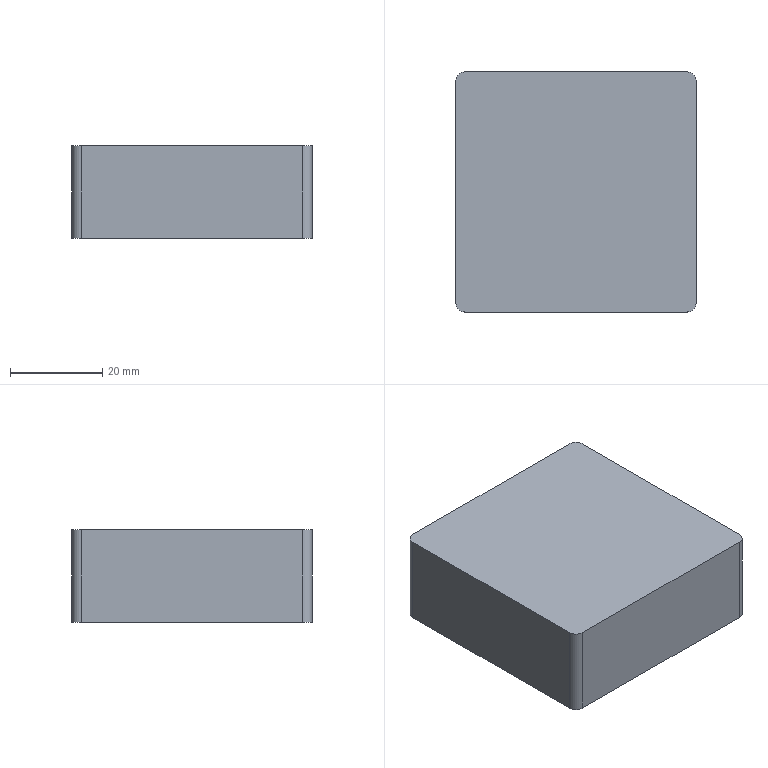Part | NX | features solid 2 | 1 solid | 12 faces | box 52 x 52 x 20 mm | volume 53088 mm3 | plane 7 | cylinder 5 | commonest cylinder face diameters 4 x4 14 x1
STEP:
#1=CARTESIAN_POINT('',(229.,-34.,-110.));
#2=VERTEX_POINT('',#1);
#3=CARTESIAN_POINT('',(229.,14.,-110.));
#4=VERTEX_POINT('',#3);
#5=CARTESIAN_POINT('',(229.,-40.,-110.));
#6=DIRECTION('',(0.,1.,0.));
#7=VECTOR('',#6,1000.);
#8=LINE('',#5,#7);
#9=EDGE_CURVE('',#2,#4,#8,.T.);
#10=ORIENTED_EDGE('',*,*,#9,.F.);
#11=CARTESIAN_POINT('',(229.,-34.,-90.));
#12=VERTEX_POINT('',#11);
#13=CARTESIAN_POINT('',(229.,-34.,-110.));
#14=DIRECTION('',(0.,0.,1.));
#15=VECTOR('',#14,1000.);
#16=LINE('',#13,#15);
#17=EDGE_CURVE('',#2,#12,#16,.T.);
#18=ORIENTED_EDGE('',*,*,#17,.T.);
#19=CARTESIAN_POINT('',(229.,14.,-90.));
#20=VERTEX_POINT('',#19);
#21=CARTESIAN_POINT('',(229.,-40.,-90.));
#22=DIRECTION('',(0.,1.,0.));
#23=VECTOR('',#22,1000.);
#24=LINE('',#21,#23);
#25=EDGE_CURVE('',#12,#20,#24,.T.);
#26=ORIENTED_EDGE('',*,*,#25,.T.);
#27=CARTESIAN_POINT('',(229.,14.,-110.));
#28=DIRECTION('',(0.,0.,1.));
#29=VECTOR('',#28,1000.);
#30=LINE('',#27,#29);
#31=EDGE_CURVE('',#20,#4,#30,.F.);
#32=ORIENTED_EDGE('',*,*,#31,.T.);
#33=EDGE_LOOP('',(#10,#18,#26,#32));
#34=FACE_BOUND('',#33,.T.);
#35=CARTESIAN_POINT('',(229.,-40.,-110.));
#36=DIRECTION('',(1.,0.,0.));
#37=DIRECTION('',(0.,1.,0.));
#38=AXIS2_PLACEMENT_3D('',#35,#36,#37);
#39=PLANE('',#38);
#40=ADVANCED_FACE('',(#34),#39,.F.);
#41=CARTESIAN_POINT('',(231.,16.,-90.));
#42=VERTEX_POINT('',#41);
#43=CARTESIAN_POINT('',(279.,16.,-90.));
#44=VERTEX_POINT('',#43);
#45=CARTESIAN_POINT('',(225.,16.,-90.));
#46=DIRECTION('',(1.,0.,0.));
#47=VECTOR('',#46,1000.);
#48=LINE('',#45,#47);
#49=EDGE_CURVE('',#42,#44,#48,.T.);
#50=ORIENTED_EDGE('',*,*,#49,.T.);
#51=CARTESIAN_POINT('',(279.,16.,-110.));
#52=VERTEX_POINT('',#51);
#53=CARTESIAN_POINT('',(279.,16.,-110.));
#54=DIRECTION('',(0.,0.,1.));
#55=VECTOR('',#54,1000.);
#56=LINE('',#53,#55);
#57=EDGE_CURVE('',#44,#52,#56,.F.);
#58=ORIENTED_EDGE('',*,*,#57,.T.);
#59=CARTESIAN_POINT('',(231.,16.,-110.));
#60=VERTEX_POINT('',#59);
#61=CARTESIAN_POINT('',(225.,16.,-110.));
#62=DIRECTION('',(1.,0.,0.));
#63=VECTOR('',#62,1000.);
#64=LINE('',#61,#63);
#65=EDGE_CURVE('',#60,#52,#64,.T.);
#66=ORIENTED_EDGE('',*,*,#65,.F.);
#67=CARTESIAN_POINT('',(231.,16.,-110.));
#68=DIRECTION('',(0.,0.,1.));
#69=VECTOR('',#68,1000.);
#70=LINE('',#67,#69);
#71=EDGE_CURVE('',#60,#42,#70,.T.);
#72=ORIENTED_EDGE('',*,*,#71,.T.);
#73=EDGE_LOOP('',(#50,#58,#66,#72));
#74=FACE_BOUND('',#73,.T.);
#75=CARTESIAN_POINT('',(225.,16.,-110.));
#76=DIRECTION('',(0.,-1.,0.));
#77=DIRECTION('',(1.,0.,0.));
#78=AXIS2_PLACEMENT_3D('',#75,#76,#77);
#79=PLANE('',#78);
#80=ADVANCED_FACE('',(#74),#79,.F.);
#81=CARTESIAN_POINT('',(281.,-10.,-107.871));
#82=VERTEX_POINT('',#81);
#83=CARTESIAN_POINT('',(281.,-10.,-100.871));
#84=DIRECTION('',(-1.,0.,0.));
#85=DIRECTION('',(0.,0.,-1.));
#86=AXIS2_PLACEMENT_3D('',#83,#84,#85);
#87=CIRCLE('',#86,7.);
#88=EDGE_CURVE('',#82,#82,#87,.F.);
#89=ORIENTED_EDGE('',*,*,#88,.F.);
#90=EDGE_LOOP('',(#89));
#91=FACE_BOUND('',#90,.T.);
#92=CARTESIAN_POINT('',(281.,14.,-90.));
#93=VERTEX_POINT('',#92);
#94=CARTESIAN_POINT('',(281.,-34.,-90.));
#95=VERTEX_POINT('',#94);
#96=CARTESIAN_POINT('',(281.,20.,-90.));
#97=DIRECTION('',(0.,-1.,0.));
#98=VECTOR('',#97,1000.);
#99=LINE('',#96,#98);
#100=EDGE_CURVE('',#93,#95,#99,.T.);
#101=ORIENTED_EDGE('',*,*,#100,.T.);
#102=CARTESIAN_POINT('',(281.,-34.,-110.));
#103=VERTEX_POINT('',#102);
#104=CARTESIAN_POINT('',(281.,-34.,-110.));
#105=DIRECTION('',(0.,0.,1.));
#106=VECTOR('',#105,1000.);
#107=LINE('',#104,#106);
#108=EDGE_CURVE('',#95,#103,#107,.F.);
#109=ORIENTED_EDGE('',*,*,#108,.T.);
#110=CARTESIAN_POINT('',(281.,14.,-110.));
#111=VERTEX_POINT('',#110);
#112=CARTESIAN_POINT('',(281.,20.,-110.));
#113=DIRECTION('',(0.,-1.,0.));
#114=VECTOR('',#113,1000.);
#115=LINE('',#112,#114);
#116=EDGE_CURVE('',#111,#103,#115,.T.);
#117=ORIENTED_EDGE('',*,*,#116,.F.);
#118=CARTESIAN_POINT('',(281.,14.,-110.));
#119=DIRECTION('',(0.,0.,1.));
#120=VECTOR('',#119,1000.);
#121=LINE('',#118,#120);
#122=EDGE_CURVE('',#111,#93,#121,.T.);
#123=ORIENTED_EDGE('',*,*,#122,.T.);
#124=EDGE_LOOP('',(#101,#109,#117,#123));
#125=FACE_BOUND('',#124,.T.);
#126=CARTESIAN_POINT('',(281.,20.,-110.));
#127=DIRECTION('',(-1.,0.,0.));
#128=DIRECTION('',(0.,0.,-1.));
#129=AXIS2_PLACEMENT_3D('',#126,#127,#128);
#130=PLANE('',#129);
#131=ADVANCED_FACE('',(#91,#125),#130,.F.);
#132=CARTESIAN_POINT('',(279.,-36.,-110.));
#133=VERTEX_POINT('',#132);
#134=CARTESIAN_POINT('',(231.,-36.,-110.));
#135=VERTEX_POINT('',#134);
#136=CARTESIAN_POINT('',(285.,-36.,-110.));
#137=DIRECTION('',(-1.,0.,0.));
#138=VECTOR('',#137,1000.);
#139=LINE('',#136,#138);
#140=EDGE_CURVE('',#133,#135,#139,.T.);
#141=ORIENTED_EDGE('',*,*,#140,.F.);
#142=CARTESIAN_POINT('',(279.,-36.,-90.));
#143=VERTEX_POINT('',#142);
#144=CARTESIAN_POINT('',(279.,-36.,-110.));
#145=DIRECTION('',(0.,0.,1.));
#146=VECTOR('',#145,1000.);
#147=LINE('',#144,#146);
#148=EDGE_CURVE('',#133,#143,#147,.T.);
#149=ORIENTED_EDGE('',*,*,#148,.T.);
#150=CARTESIAN_POINT('',(231.,-36.,-90.));
#151=VERTEX_POINT('',#150);
#152=CARTESIAN_POINT('',(285.,-36.,-90.));
#153=DIRECTION('',(-1.,0.,0.));
#154=VECTOR('',#153,1000.);
#155=LINE('',#152,#154);
#156=EDGE_CURVE('',#143,#151,#155,.T.);
#157=ORIENTED_EDGE('',*,*,#156,.T.);
#158=CARTESIAN_POINT('',(231.,-36.,-110.));
#159=DIRECTION('',(0.,0.,1.));
#160=VECTOR('',#159,1000.);
#161=LINE('',#158,#160);
#162=EDGE_CURVE('',#151,#135,#161,.F.);
#163=ORIENTED_EDGE('',*,*,#162,.T.);
#164=EDGE_LOOP('',(#141,#149,#157,#163));
#165=FACE_BOUND('',#164,.T.);
#166=CARTESIAN_POINT('',(285.,-36.,-110.));
#167=DIRECTION('',(0.,1.,0.));
#168=DIRECTION('',(0.,0.,1.));
#169=AXIS2_PLACEMENT_3D('',#166,#167,#168);
#170=PLANE('',#169);
#171=ADVANCED_FACE('',(#165),#170,.F.);
#172=ORIENTED_EDGE('',*,*,#116,.T.);
#173=CARTESIAN_POINT('',(279.,-34.,-110.));
#174=DIRECTION('',(0.,0.,-1.));
#175=DIRECTION('',(0.,1.,0.));
#176=AXIS2_PLACEMENT_3D('',#173,#174,#175);
#177=CIRCLE('',#176,2.);
#178=EDGE_CURVE('',#103,#133,#177,.T.);
#179=ORIENTED_EDGE('',*,*,#178,.T.);
#180=ORIENTED_EDGE('',*,*,#140,.T.);
#181=CARTESIAN_POINT('',(231.,-34.,-110.));
#182=DIRECTION('',(0.,0.,-1.));
#183=DIRECTION('',(0.,1.,0.));
#184=AXIS2_PLACEMENT_3D('',#181,#182,#183);
#185=CIRCLE('',#184,2.);
#186=EDGE_CURVE('',#135,#2,#185,.T.);
#187=ORIENTED_EDGE('',*,*,#186,.T.);
#188=ORIENTED_EDGE('',*,*,#9,.T.);
#189=CARTESIAN_POINT('',(231.,14.,-110.));
#190=DIRECTION('',(0.,0.,-1.));
#191=DIRECTION('',(0.,1.,0.));
#192=AXIS2_PLACEMENT_3D('',#189,#190,#191);
#193=CIRCLE('',#192,2.);
#194=EDGE_CURVE('',#4,#60,#193,.T.);
#195=ORIENTED_EDGE('',*,*,#194,.T.);
#196=ORIENTED_EDGE('',*,*,#65,.T.);
#197=CARTESIAN_POINT('',(279.,14.,-110.));
#198=DIRECTION('',(0.,0.,-1.));
#199=DIRECTION('',(0.,1.,0.));
#200=AXIS2_PLACEMENT_3D('',#197,#198,#199);
#201=CIRCLE('',#200,2.);
#202=EDGE_CURVE('',#52,#111,#201,.T.);
#203=ORIENTED_EDGE('',*,*,#202,.T.);
#204=EDGE_LOOP('',(#172,#179,#180,#187,#188,#195,#196,#203));
#205=FACE_BOUND('',#204,.T.);
#206=CARTESIAN_POINT('',(225.,20.,-110.));
#207=DIRECTION('',(0.,0.,-1.));
#208=DIRECTION('',(0.,1.,0.));
#209=AXIS2_PLACEMENT_3D('',#206,#207,#208);
#210=PLANE('',#209);
#211=ADVANCED_FACE('',(#205),#210,.T.);
#212=ORIENTED_EDGE('',*,*,#156,.F.);
#213=CARTESIAN_POINT('',(279.,-34.,-90.));
#214=DIRECTION('',(0.,0.,-1.));
#215=DIRECTION('',(0.,1.,0.));
#216=AXIS2_PLACEMENT_3D('',#213,#214,#215);
#217=CIRCLE('',#216,2.);
#218=EDGE_CURVE('',#143,#95,#217,.F.);
#219=ORIENTED_EDGE('',*,*,#218,.T.);
#220=ORIENTED_EDGE('',*,*,#100,.F.);
#221=CARTESIAN_POINT('',(279.,14.,-90.));
#222=DIRECTION('',(0.,0.,-1.));
#223=DIRECTION('',(0.,1.,0.));
#224=AXIS2_PLACEMENT_3D('',#221,#222,#223);
#225=CIRCLE('',#224,2.);
#226=EDGE_CURVE('',#93,#44,#225,.F.);
#227=ORIENTED_EDGE('',*,*,#226,.T.);
#228=ORIENTED_EDGE('',*,*,#49,.F.);
#229=CARTESIAN_POINT('',(231.,14.,-90.));
#230=DIRECTION('',(0.,0.,-1.));
#231=DIRECTION('',(0.,1.,0.));
#232=AXIS2_PLACEMENT_3D('',#229,#230,#231);
#233=CIRCLE('',#232,2.);
#234=EDGE_CURVE('',#42,#20,#233,.F.);
#235=ORIENTED_EDGE('',*,*,#234,.T.);
#236=ORIENTED_EDGE('',*,*,#25,.F.);
#237=CARTESIAN_POINT('',(231.,-34.,-90.));
#238=DIRECTION('',(0.,0.,-1.));
#239=DIRECTION('',(0.,1.,0.));
#240=AXIS2_PLACEMENT_3D('',#237,#238,#239);
#241=CIRCLE('',#240,2.);
#242=EDGE_CURVE('',#12,#151,#241,.F.);
#243=ORIENTED_EDGE('',*,*,#242,.T.);
#244=EDGE_LOOP('',(#212,#219,#220,#227,#228,#235,#236,#243));
#245=FACE_BOUND('',#244,.T.);
#246=CARTESIAN_POINT('',(225.,20.,-90.));
#247=DIRECTION('',(0.,0.,-1.));
#248=DIRECTION('',(0.,1.,0.));
#249=AXIS2_PLACEMENT_3D('',#246,#247,#248);
#250=PLANE('',#249);
#251=ADVANCED_FACE('',(#245),#250,.F.);
#252=CARTESIAN_POINT('',(275.,-17.,-100.871));
#253=VERTEX_POINT('',#252);
#254=CARTESIAN_POINT('',(275.,-10.,-100.871));
#255=DIRECTION('',(1.,0.,0.));
#256=DIRECTION('',(0.,-1.,0.));
#257=AXIS2_PLACEMENT_3D('',#254,#255,#256);
#258=CIRCLE('',#257,7.);
#259=EDGE_CURVE('',#253,#253,#258,.T.);
#260=ORIENTED_EDGE('',*,*,#259,.F.);
#261=EDGE_LOOP('',(#260));
#262=FACE_BOUND('',#261,.T.);
#263=ORIENTED_EDGE('',*,*,#88,.T.);
#264=EDGE_LOOP('',(#263));
#265=FACE_BOUND('',#264,.T.);
#266=CARTESIAN_POINT('',(275.,-10.,-100.871));
#267=DIRECTION('',(1.,0.,0.));
#268=DIRECTION('',(0.,0.,1.));
#269=AXIS2_PLACEMENT_3D('',#266,#267,#268);
#270=CYLINDRICAL_SURFACE('',#269,7.);
#271=ADVANCED_FACE('',(#262,#265),#270,.F.);
#272=ORIENTED_EDGE('',*,*,#259,.T.);
#273=EDGE_LOOP('',(#272));
#274=FACE_BOUND('',#273,.T.);
#275=CARTESIAN_POINT('',(275.,-10.,-100.871));
#276=DIRECTION('',(1.,0.,0.));
#277=DIRECTION('',(0.,0.,1.));
#278=AXIS2_PLACEMENT_3D('',#275,#276,#277);
#279=PLANE('',#278);
#280=ADVANCED_FACE('',(#274),#279,.T.);
#281=ORIENTED_EDGE('',*,*,#178,.F.);
#282=ORIENTED_EDGE('',*,*,#108,.F.);
#283=ORIENTED_EDGE('',*,*,#218,.F.);
#284=ORIENTED_EDGE('',*,*,#148,.F.);
#285=EDGE_LOOP('',(#281,#282,#283,#284));
#286=FACE_BOUND('',#285,.T.);
#287=CARTESIAN_POINT('',(279.,-34.,-110.));
#288=DIRECTION('',(0.,0.,1.));
#289=DIRECTION('',(0.,-1.,0.));
#290=AXIS2_PLACEMENT_3D('',#287,#288,#289);
#291=CYLINDRICAL_SURFACE('',#290,2.);
#292=ADVANCED_FACE('',(#286),#291,.T.);
#293=ORIENTED_EDGE('',*,*,#186,.F.);
#294=ORIENTED_EDGE('',*,*,#162,.F.);
#295=ORIENTED_EDGE('',*,*,#242,.F.);
#296=ORIENTED_EDGE('',*,*,#17,.F.);
#297=EDGE_LOOP('',(#293,#294,#295,#296));
#298=FACE_BOUND('',#297,.T.);
#299=CARTESIAN_POINT('',(231.,-34.,-110.));
#300=DIRECTION('',(0.,0.,1.));
#301=DIRECTION('',(0.,-1.,0.));
#302=AXIS2_PLACEMENT_3D('',#299,#300,#301);
#303=CYLINDRICAL_SURFACE('',#302,2.);
#304=ADVANCED_FACE('',(#298),#303,.T.);
#305=ORIENTED_EDGE('',*,*,#202,.F.);
#306=ORIENTED_EDGE('',*,*,#57,.F.);
#307=ORIENTED_EDGE('',*,*,#226,.F.);
#308=ORIENTED_EDGE('',*,*,#122,.F.);
#309=EDGE_LOOP('',(#305,#306,#307,#308));
#310=FACE_BOUND('',#309,.T.);
#311=CARTESIAN_POINT('',(279.,14.,-110.));
#312=DIRECTION('',(0.,0.,1.));
#313=DIRECTION('',(0.,-1.,0.));
#314=AXIS2_PLACEMENT_3D('',#311,#312,#313);
#315=CYLINDRICAL_SURFACE('',#314,2.);
#316=ADVANCED_FACE('',(#310),#315,.T.);
#317=ORIENTED_EDGE('',*,*,#194,.F.);
#318=ORIENTED_EDGE('',*,*,#31,.F.);
#319=ORIENTED_EDGE('',*,*,#234,.F.);
#320=ORIENTED_EDGE('',*,*,#71,.F.);
#321=EDGE_LOOP('',(#317,#318,#319,#320));
#322=FACE_BOUND('',#321,.T.);
#323=CARTESIAN_POINT('',(231.,14.,-110.));
#324=DIRECTION('',(0.,0.,1.));
#325=DIRECTION('',(0.,-1.,0.));
#326=AXIS2_PLACEMENT_3D('',#323,#324,#325);
#327=CYLINDRICAL_SURFACE('',#326,2.);
#328=ADVANCED_FACE('',(#322),#327,.T.);
#329=CLOSED_SHELL('',(#40,#80,#131,#171,#211,#251,#271,#280,#292,#304,#316,#328));
#330=MANIFOLD_SOLID_BREP('',#329);
#331=(LENGTH_UNIT()NAMED_UNIT(*)SI_UNIT(.MILLI.,.METRE.));
#332=UNCERTAINTY_MEASURE_WITH_UNIT(LENGTH_MEASURE(0.00001),#331,'','');
#333=(NAMED_UNIT(*)PLANE_ANGLE_UNIT()SI_UNIT($,.RADIAN.));
#334=(NAMED_UNIT(*)SI_UNIT($,.STERADIAN.)SOLID_ANGLE_UNIT());
#335=(GEOMETRIC_REPRESENTATION_CONTEXT(3)GLOBAL_UNCERTAINTY_ASSIGNED_CONTEXT((#332))GLOBAL_UNIT_ASSIGNED_CONTEXT((#331,#333,#334))REPRESENTATION_CONTEXT('',''));
#336=ADVANCED_BREP_SHAPE_REPRESENTATION('',(#330),#335);